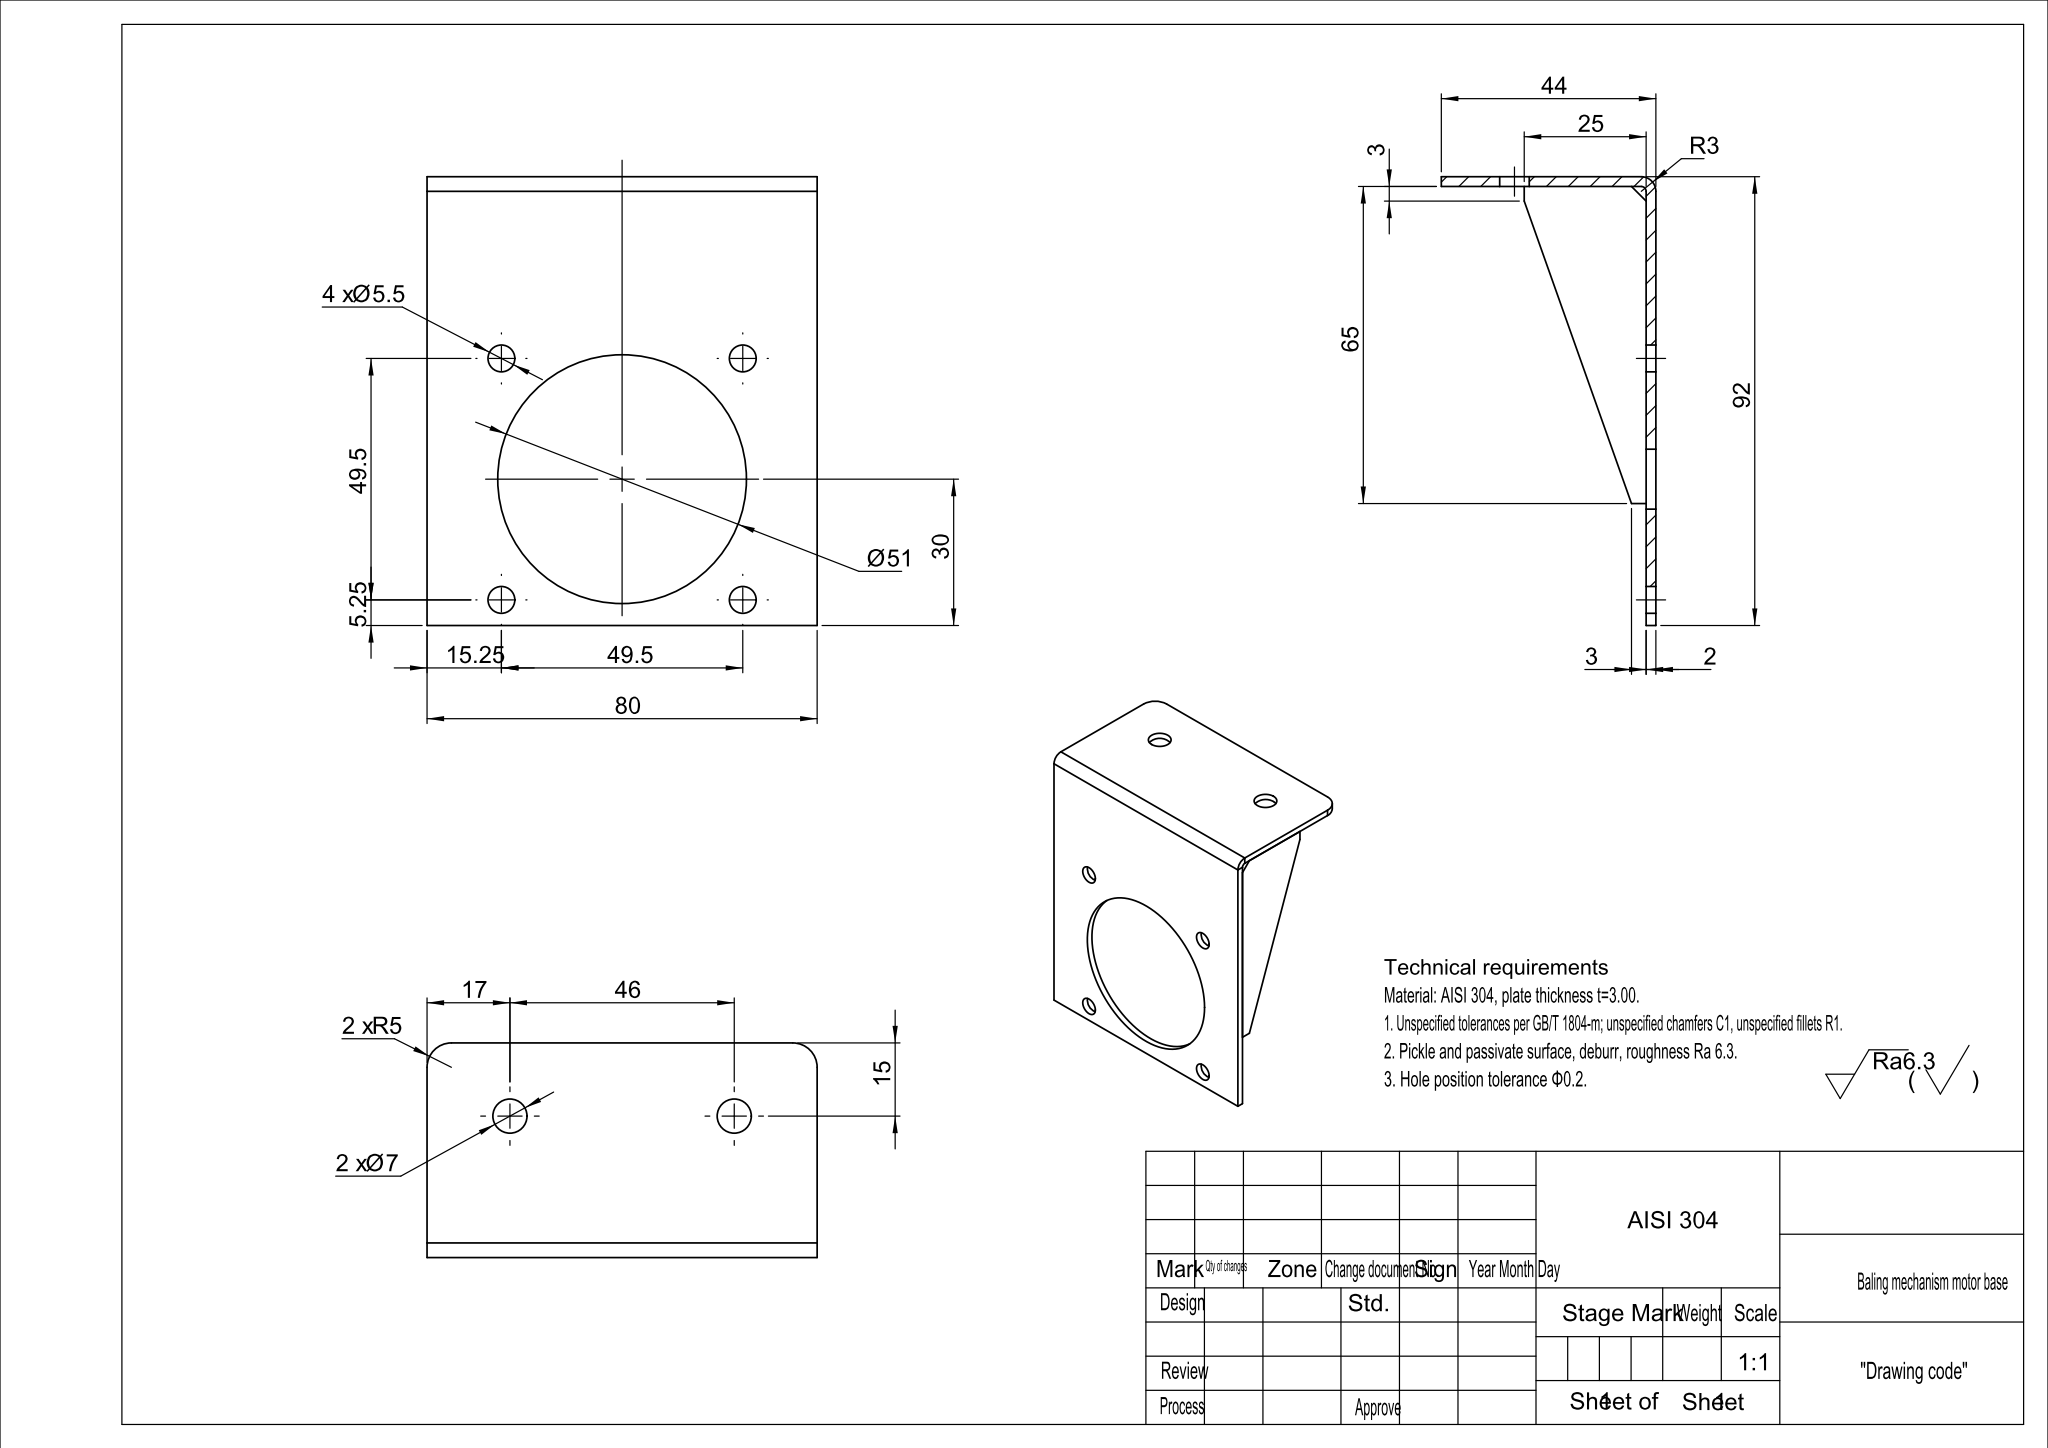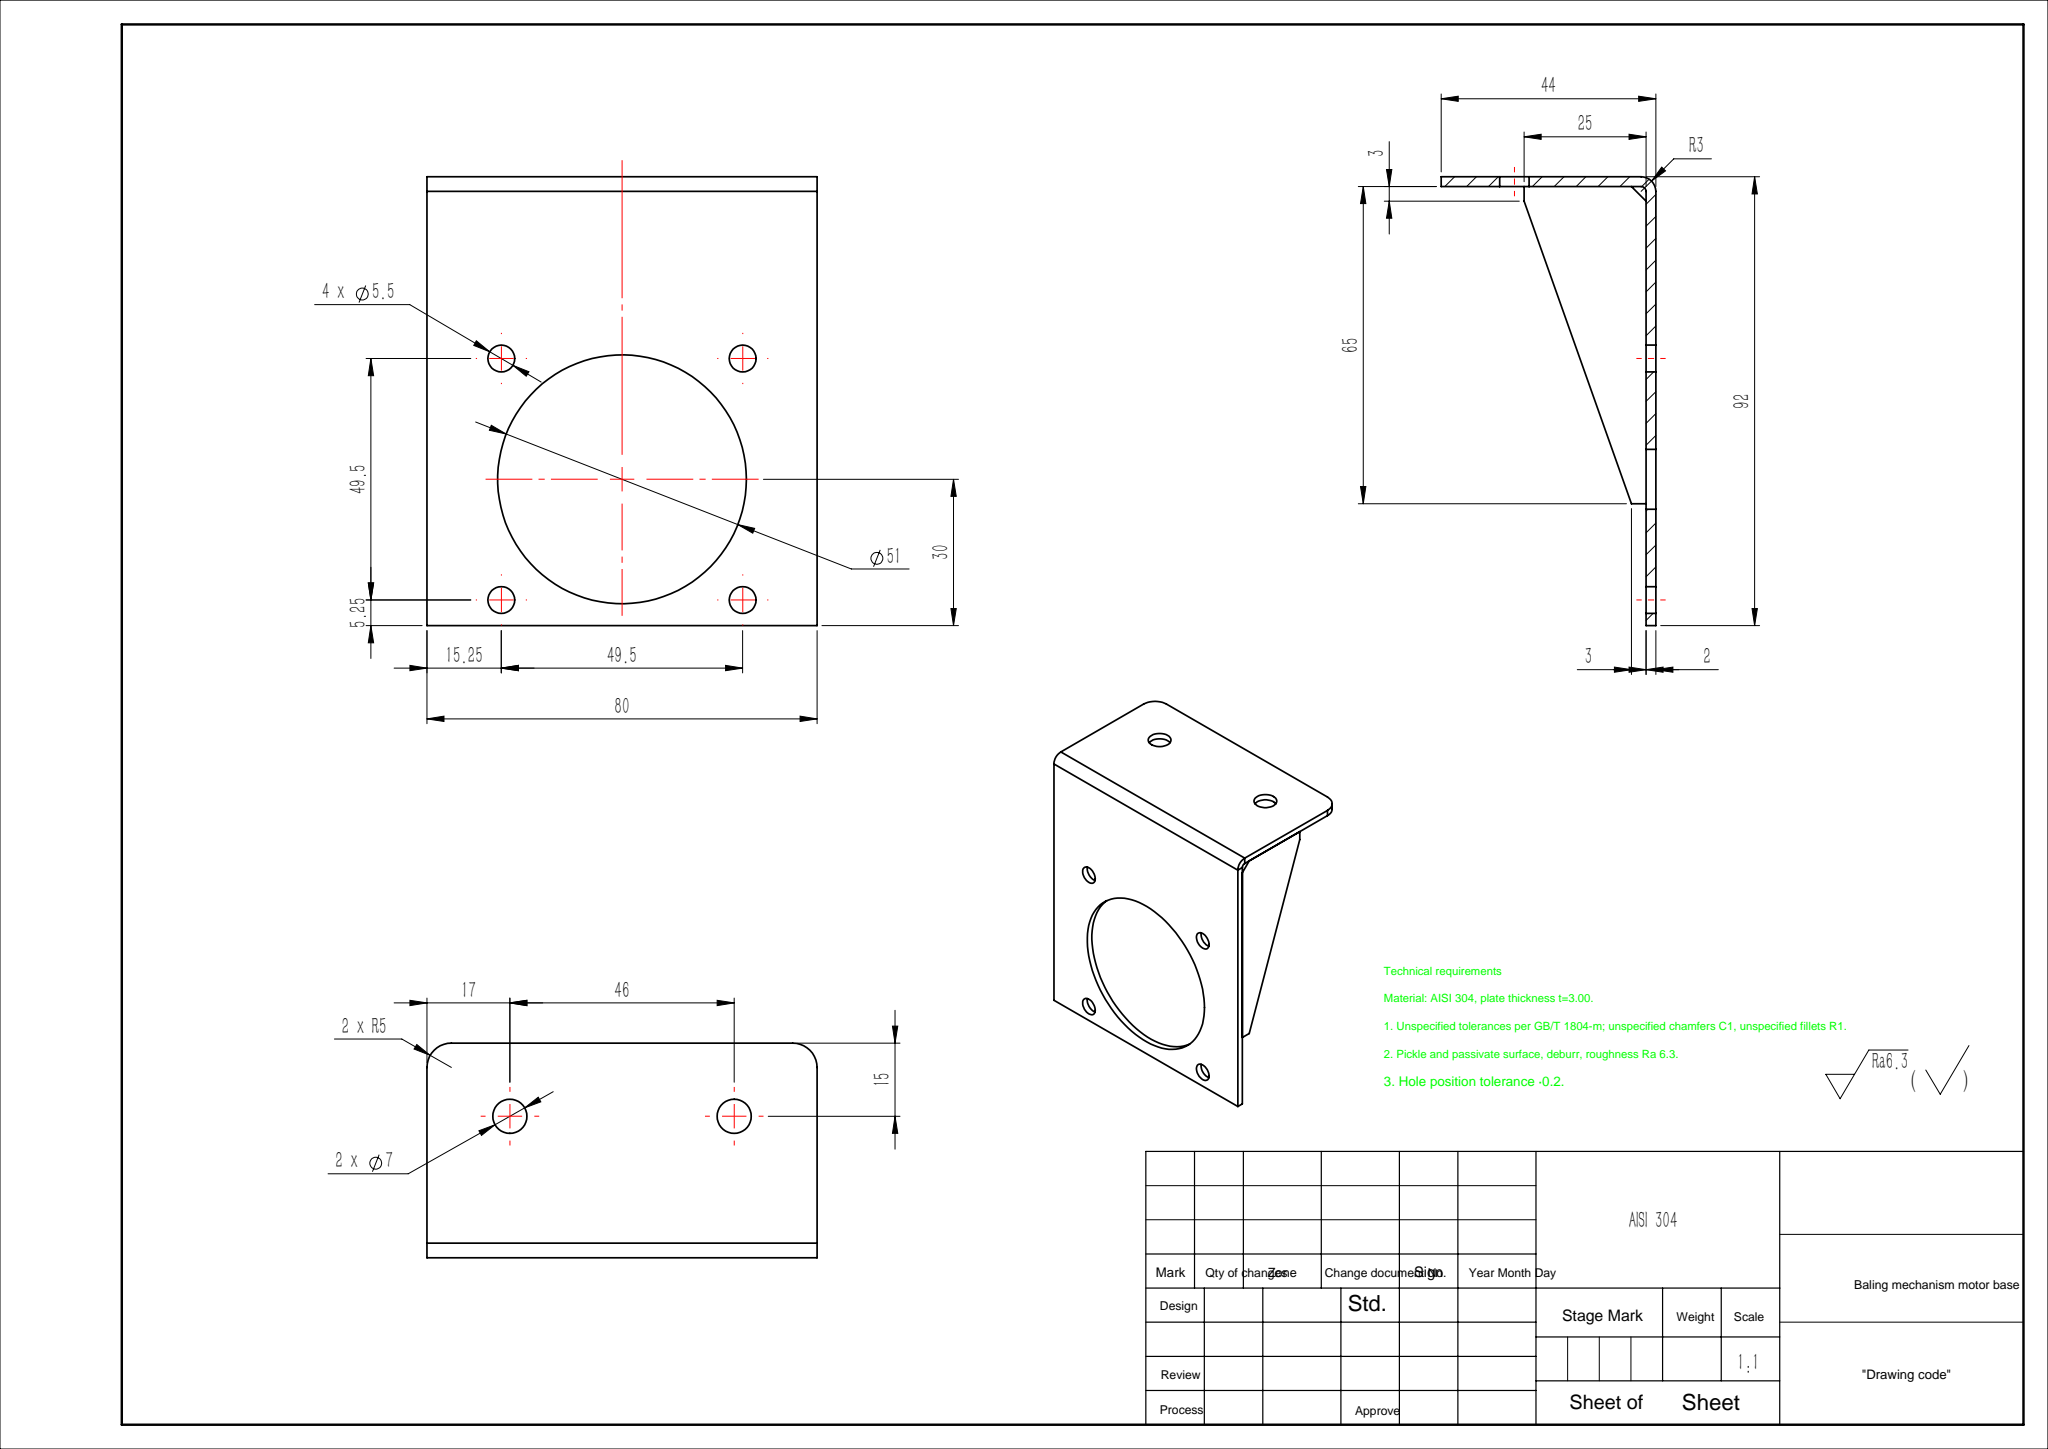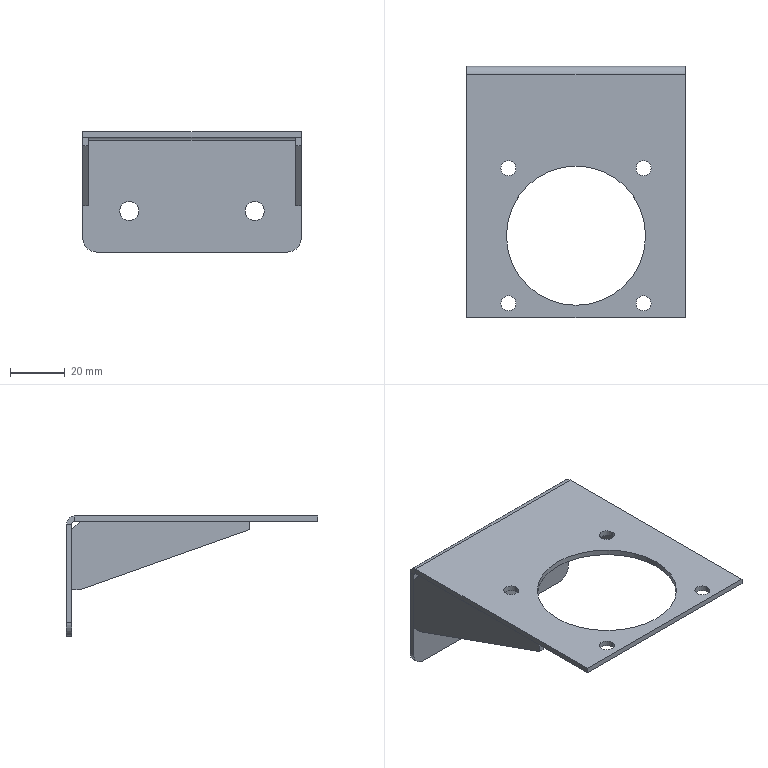Part | SolidWorks | features Gusset 2, EdgeFlange 1, Fillet 1, FlatPattern 1, ICE 1, SMBaseFlange 1, SheetMetal 1 | 3 solids | 46 faces | box 80 x 92 x 44 mm | volume 20606 mm3 | plane 28 | cylinder 18 | commonest cylinder face diameters 5.5 x8 7 x4 10 x2 51 x2 2 x1 6 x1